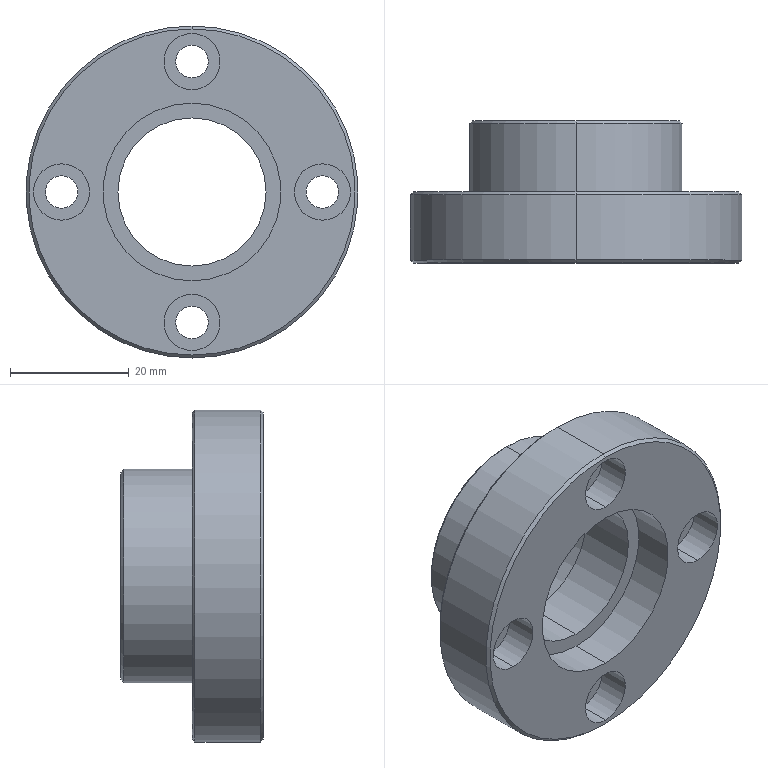Part | STEP file | QA-FC10 | 1 solid | 41 faces | box 56 x 24 x 56 mm | volume 24731 mm3 | cylinder 26 | plane 9 | cone 6 | commonest cylinder face diameters 5.5 x8 9.5 x8 30 x4 25 x2 36 x2 56 x2